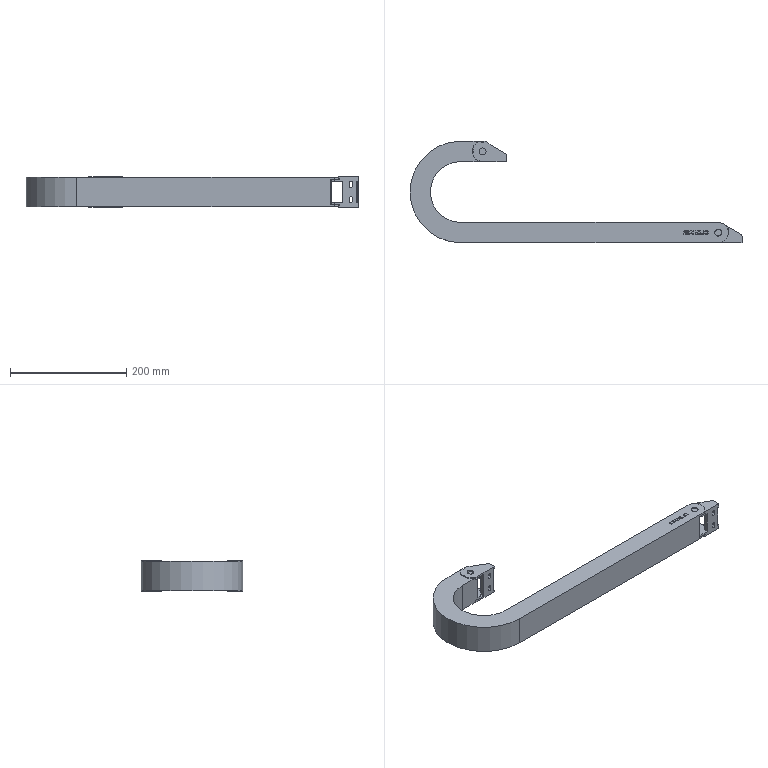Part | SolidWorks | features BaseBody 3 | 3 solids | 226 faces | box 572.2 x 175 x 53 mm | volume 617417 mm3 | plane 134 | cylinder 84 | spline 8 | commonest cylinder face diameters 35 x23 12 x16 6.2 x12 1 x8 1.407 x4 2.982 x4